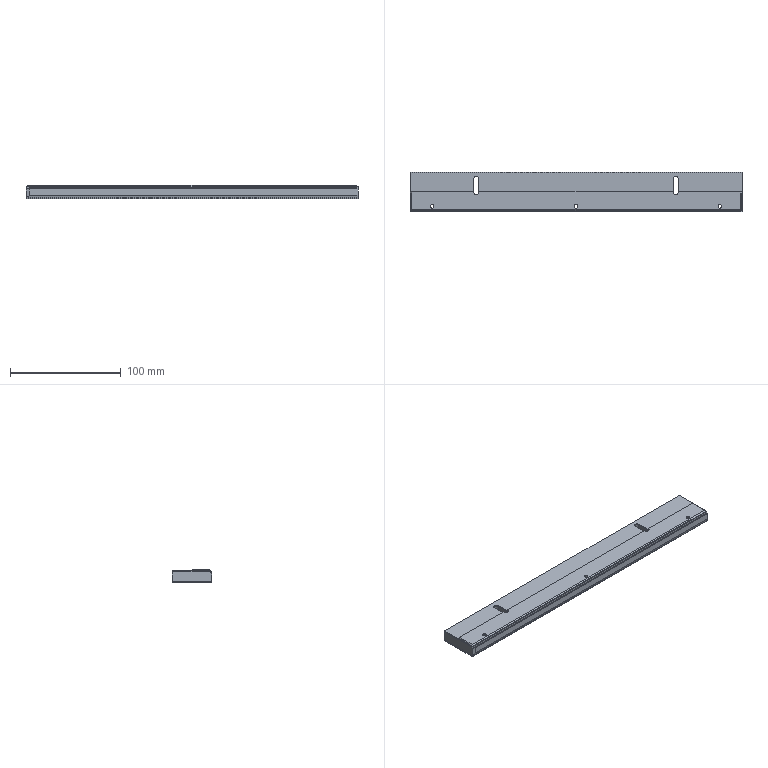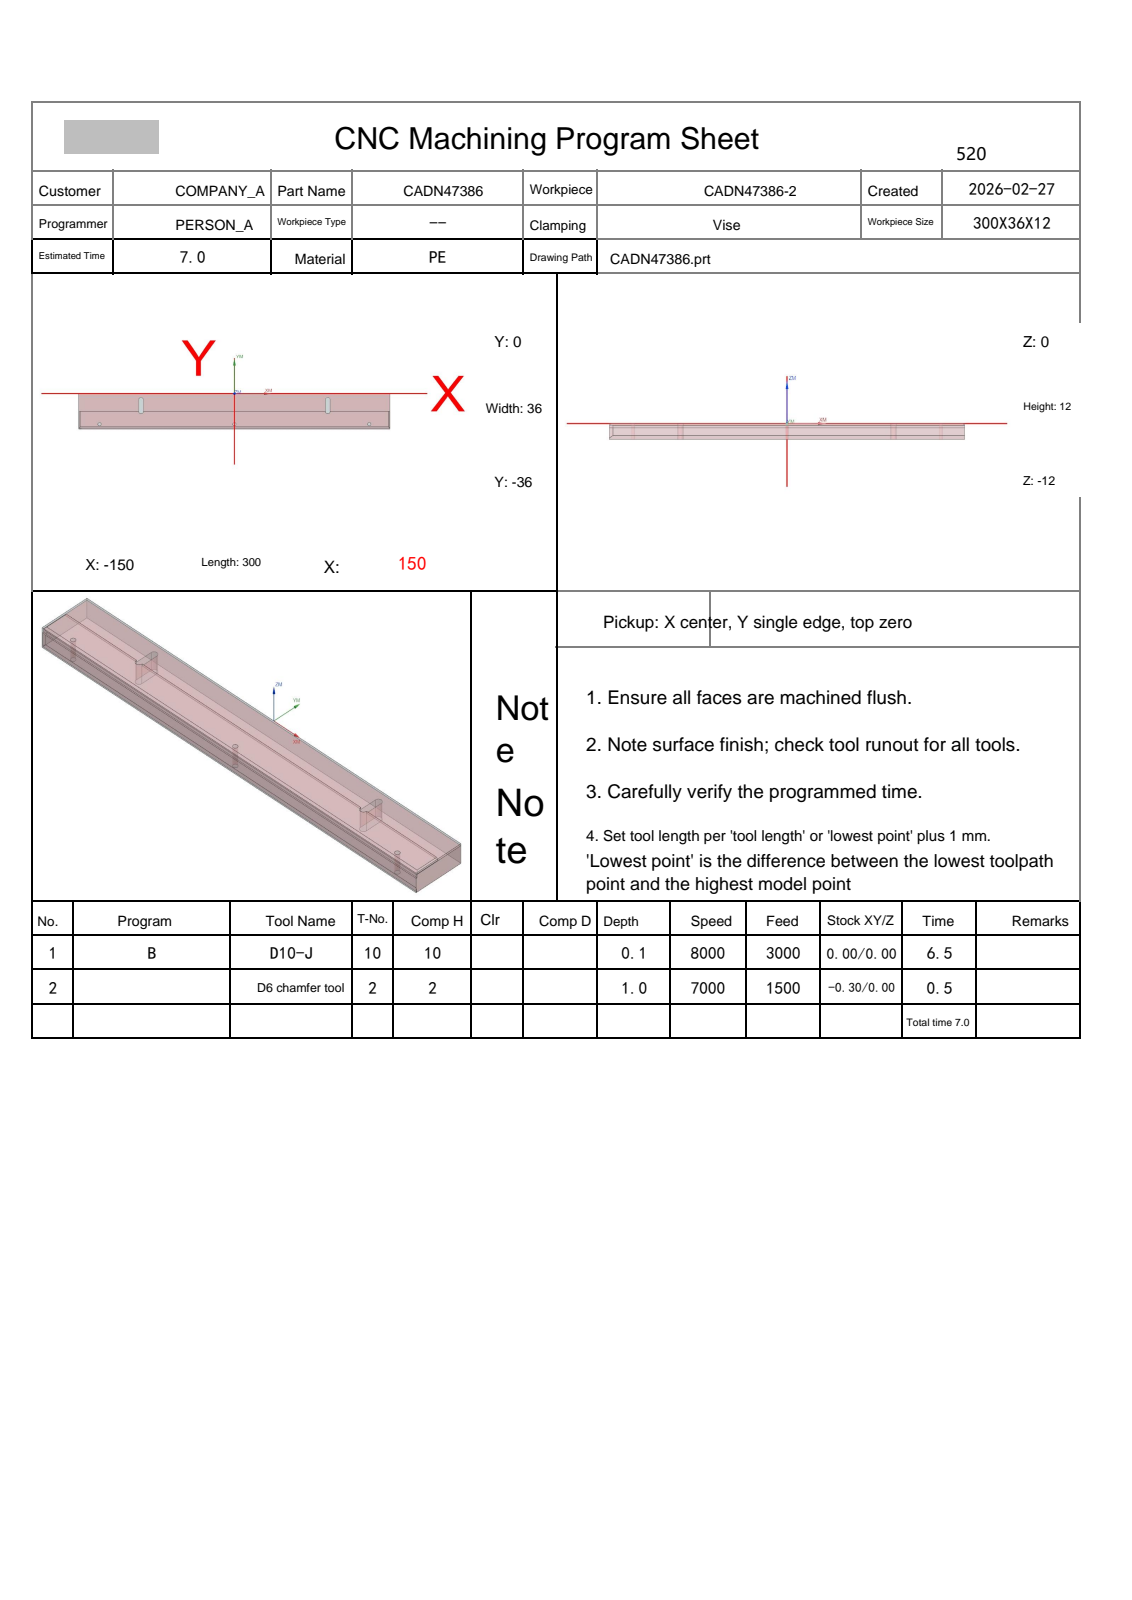NC program | NX | posted by the shop | part box 300 x 36 x 12 mm
Whole program:
%
O0001
(Machine time: 7.37 MIN)
(===Total Tool:2===)
(T10=D10-J  D=10.  R=0.   D-  H10 Z=0.    )
(T2=D6 chamfer tool   D=6.   R=0.   D-  H02 Z=-1.   )
G80 G90 G17 G49 G40
G91 G28 Z0
M01
N1 T10 M06
(D10-J  D=10. R=0. H=10 ce=0.20 di=0.10)
G00 G90 G54 X133.111 Y17. M03 S8000
G43 H10 Z50.
M08
Z4.02
G01 Z2.02 F3000.
X145.111 Y5.
X154.707 Y-4.596
G02 X155. Y-5.303 I-.707 J-.707
G01 Y-13.812
G02 X154.6 Y-14.212 I-.4 J0.0
X154.317 Y-14.095 I0.0 J.4
G01 X135.515 Y4.707
G03 X134.808 Y5. I-.707 J-.707
G01 X126.299
G03 X125.899 Y4.6 I0.0 J-.4
X126.016 Y4.317 I.4 J0.0
G01 X154.707 Y-24.374
G02 X155. Y-25.08 I-.707 J-.707
G01 Y-33.59
G02 X154.6 Y-33.99 I-.4 J0.0
X154.317 Y-33.873 I0.0 J.4
G01 X115.737 Y4.707
G03 X115.031 Y5. I-.707 J-.707
G01 X106.521
G03 X106.121 Y4.6 I0.0 J-.4
X106.238 Y4.317 I.4 J0.0
G01 X150.873 Y-40.317
G02 X150.99 Y-40.6 I-.283 J-.283
X150.59 Y-41. I-.4 J0.0
G01 X142.08
G02 X141.374 Y-40.707 I.001 J1.
G01 X95.959 Y4.707
G03 X95.253 Y5. I-.707 J-.707
G01 X86.743
G03 X86.343 Y4.6 I0.0 J-.4
X86.46 Y4.317 I.4 J0.0
G01 X131.095 Y-40.317
G02 X131.212 Y-40.6 I-.283 J-.283
X130.812 Y-41. I-.4 J0.0
G01 X122.303
G02 X121.596 Y-40.707 I.001 J1.
G01 X76.181 Y4.707
G03 X75.475 Y5. I-.707 J-.707
G01 X66.965
G03 X66.566 Y4.6 I0.0 J-.4
X66.683 Y4.317 I.4 J0.0
G01 X111.317 Y-40.317
G02 X111.434 Y-40.6 I-.283 J-.283
X111.035 Y-41. I-.4 J0.0
G01 X102.525
G02 X101.819 Y-40.707 I.001 J1.
G01 X56.404 Y4.707
G03 X55.697 Y5. I-.707 J-.707
G01 X47.188
G03 X46.788 Y4.6 I0.0 J-.4
X46.905 Y4.317 I.4 J0.0
G01 X91.54 Y-40.317
G02 X91.657 Y-40.6 I-.283 J-.283
X91.257 Y-41. I-.4 J0.0
G01 X82.747
G02 X82.041 Y-40.707 I.001 J1.
G01 X36.626 Y4.707
G03 X35.92 Y5. I-.707 J-.707
G01 X27.41
G03 X27.01 Y4.6 I0.0 J-.4
X27.127 Y4.317 I.4 J0.0
G01 X71.762 Y-40.317
G02 X71.879 Y-40.6 I-.283 J-.283
X71.479 Y-41. I-.4 J0.0
G01 X62.969
G02 X62.263 Y-40.707 I.001 J1.
G01 X16.848 Y4.707
G03 X16.142 Y5. I-.707 J-.707
G01 X7.632
G03 X7.232 Y4.6 I0.0 J-.4
X7.349 Y4.317 I.4 J0.0
G01 X51.984 Y-40.317
G02 X52.101 Y-40.6 I-.283 J-.283
X51.701 Y-41. I-.4 J0.0
G01 X43.191
G02 X42.485 Y-40.707 I.001 J1.
G01 X-2.93 Y4.707
G03 X-3.636 Y5. I-.707 J-.707
G01 X-12.146
G03 X-12.545 Y4.6 I0.0 J-.4
X-12.429 Y4.317 I.4 J0.0
G01 X32.206 Y-40.317
G02 X32.323 Y-40.6 I-.283 J-.283
X31.924 Y-41. I-.4 J0.0
G01 X23.414
G02 X22.707 Y-40.707 I.001 J1.
G01 X-22.707 Y4.707
G03 X-23.414 Y5. I-.707 J-.707
G01 X-31.924
G03 X-32.323 Y4.6 I0.0 J-.4
X-32.206 Y4.317 I.4 J0.0
G01 X12.429 Y-40.317
G02 X12.545 Y-40.6 I-.283 J-.283
X12.146 Y-41. I-.4 J0.0
G01 X3.636
G02 X2.93 Y-40.708 I.001 J1.
G01 X-42.485 Y4.707
G03 X-43.191 Y5. I-.707 J-.707
G01 X-51.701
G03 X-52.101 Y4.6 I0.0 J-.4
X-51.984 Y4.317 I.4 J0.0
G01 X-7.349 Y-40.317
G02 X-7.232 Y-40.6 I-.283 J-.283
X-7.632 Y-41. I-.4 J0.0
G01 X-16.142
G02 X-16.848 Y-40.708 I.001 J1.
G01 X-62.263 Y4.707
G03 X-62.969 Y5. I-.707 J-.707
G01 X-71.479
G03 X-71.879 Y4.6 I0.0 J-.4
X-71.762 Y4.317 I.4 J0.0
G01 X-27.127 Y-40.317
G02 X-27.01 Y-40.6 I-.283 J-.283
X-27.41 Y-41. I-.4 J0.0
G01 X-35.92
G02 X-36.626 Y-40.708 I.001 J1.
G01 X-82.041 Y4.707
G03 X-82.747 Y5. I-.707 J-.707
G01 X-91.257
G03 X-91.657 Y4.6 I0.0 J-.4
X-91.54 Y4.317 I.4 J0.0
G01 X-46.905 Y-40.317
G02 X-46.788 Y-40.6 I-.283 J-.283
X-47.188 Y-41. I-.4 J0.0
G01 X-55.697
G02 X-56.404 Y-40.708 I.001 J1.
G01 X-101.819 Y4.707
G03 X-102.525 Y5. I-.707 J-.707
G01 X-111.035
G03 X-111.434 Y4.6 I0.0 J-.4
X-111.317 Y4.317 I.4 J0.0
G01 X-66.683 Y-40.317
G02 X-66.566 Y-40.6 I-.283 J-.283
X-66.965 Y-41. I-.4 J0.0
G01 X-75.475
G02 X-76.181 Y-40.707 I.001 J1.
G01 X-121.596 Y4.707
G03 X-122.303 Y5. I-.707 J-.707
G01 X-130.812
G03 X-131.212 Y4.6 I0.0 J-.4
X-131.095 Y4.317 I.4 J0.0
G01 X-86.46 Y-40.317
G02 X-86.343 Y-40.6 I-.283 J-.283
X-86.743 Y-41. I-.4 J0.0
G01 X-95.253
G02 X-95.959 Y-40.707 I.001 J1.
G01 X-141.374 Y4.707
G03 X-142.08 Y5. I-.707 J-.707
G01 X-150.59
G03 X-150.99 Y4.6 I0.0 J-.4
X-150.873 Y4.317 I.4 J0.0
G01 X-106.238 Y-40.317
G02 X-106.121 Y-40.6 I-.283 J-.283
X-106.521 Y-41. I-.4 J0.0
G01 X-115.031
G02 X-115.737 Y-40.707 I.001 J1.
G01 X-154.317 Y-2.127
G03 X-154.6 Y-2.01 I-.283 J-.283
X-155. Y-2.41 I0.0 J-.4
G01 Y-10.92
G03 X-154.707 Y-11.626 I1. J.001
G01 X-126.016 Y-40.317
G02 X-125.899 Y-40.6 I-.283 J-.283
X-126.299 Y-41. I-.4 J0.0
G01 X-134.808
G02 X-135.515 Y-40.707 I0.0 J1.
G01 X-154.317 Y-21.905
G03 X-154.6 Y-21.788 I-.283 J-.283
X-155. Y-22.188 I0.0 J-.4
G01 Y-30.697
G03 X-154.707 Y-31.404 I1. J0.0
G01 X-145.111 Y-41.
X-133.111 Y-53.
Z4.02
G00 Z5.5
X167. Y-16.889
Z3.54
G01 Z1.54
X155. Y-4.889
X145.404 Y4.707
G03 X144.697 Y5. I-.707 J-.707
G01 X136.188
G03 X135.788 Y4.6 I0.0 J-.4
X135.905 Y4.317 I.4 J0.0
G01 X154.707 Y-14.485
G02 X155. Y-15.192 I-.707 J-.707
G01 Y-23.701
G02 X154.6 Y-24.101 I-.4 J0.0
X154.317 Y-23.984 I0.0 J.4
G01 X125.626 Y4.707
G03 X124.92 Y5. I-.707 J-.707
G01 X116.41
G03 X116.01 Y4.6 I0.0 J-.4
X116.127 Y4.317 I.4 J0.0
G01 X154.707 Y-34.263
G02 X155. Y-34.969 I-.707 J-.707
G01 Y-40.
G02 X154. Y-41. I-1. J0.0
G01 X151.969
G02 X151.263 Y-40.708 I.001 J1.
G01 X105.848 Y4.707
G03 X105.142 Y5. I-.707 J-.707
G01 X96.632
G03 X96.232 Y4.6 I0.0 J-.4
X96.349 Y4.317 I.4 J0.0
G01 X140.984 Y-40.317
G02 X141.101 Y-40.6 I-.283 J-.283
X140.701 Y-41. I-.4 J0.0
G01 X132.191
G02 X131.485 Y-40.707 I.001 J1.
G01 X86.07 Y4.707
G03 X85.364 Y5. I-.707 J-.707
G01 X76.854
G03 X76.455 Y4.6 I0.0 J-.4
X76.571 Y4.317 I.4 J0.0
G01 X121.206 Y-40.317
G02 X121.323 Y-40.6 I-.283 J-.283
X120.923 Y-41. I-.4 J0.0
G01 X112.414
G02 X111.708 Y-40.708 I.001 J1.
G01 X66.293 Y4.707
G03 X65.586 Y5. I-.707 J-.707
G01 X57.076
G03 X56.677 Y4.6 I0.0 J-.4
X56.794 Y4.317 I.4 J0.0
G01 X101.429 Y-40.317
G02 X101.545 Y-40.6 I-.283 J-.283
X101.146 Y-41. I-.4 J0.0
G01 X92.636
G02 X91.93 Y-40.707 I.001 J1.
G01 X46.515 Y4.707
G03 X45.809 Y5. I-.707 J-.707
G01 X37.299
G03 X36.899 Y4.6 I0.0 J-.4
X37.016 Y4.317 I.4 J0.0
G01 X81.651 Y-40.317
G02 X81.768 Y-40.6 I-.283 J-.283
X81.368 Y-41. I-.4 J0.0
G01 X72.858
G02 X72.152 Y-40.707 I.001 J1.
G01 X26.737 Y4.707
G03 X26.031 Y5. I-.707 J-.707
G01 X17.521
G03 X17.121 Y4.6 I0.0 J-.4
X17.238 Y4.317 I.4 J0.0
G01 X61.873 Y-40.317
G02 X61.99 Y-40.6 I-.283 J-.283
X61.59 Y-41. I-.4 J0.0
G01 X53.08
G02 X52.374 Y-40.707 I.001 J1.
G01 X6.959 Y4.707
G03 X6.253 Y5. I-.707 J-.707
G01 X-2.257
G03 X-2.657 Y4.6 I0.0 J-.4
X-2.54 Y4.317 I.4 J0.0
G01 X42.095 Y-40.317
G02 X42.212 Y-40.6 I-.283 J-.283
X41.812 Y-41. I-.4 J0.0
G01 X33.303
G02 X32.596 Y-40.707 I.001 J1.
G01 X-12.819 Y4.707
G03 X-13.525 Y5. I-.707 J-.707
G01 X-22.035
G03 X-22.434 Y4.6 I0.0 J-.4
X-22.317 Y4.317 I.4 J0.0
G01 X22.317 Y-40.317
G02 X22.434 Y-40.6 I-.283 J-.283
X22.035 Y-41. I-.4 J0.0
G01 X13.525
G02 X12.819 Y-40.708 I.001 J1.
G01 X-32.596 Y4.707
G03 X-33.303 Y5. I-.707 J-.707
G01 X-41.812
G03 X-42.212 Y4.6 I0.0 J-.4
X-42.095 Y4.317 I.4 J0.0
G01 X2.54 Y-40.317
G02 X2.657 Y-40.6 I-.283 J-.283
X2.257 Y-41. I-.4 J0.0
G01 X-6.253
G02 X-6.959 Y-40.708 I.001 J1.
G01 X-52.374 Y4.707
G03 X-53.08 Y5. I-.707 J-.707
G01 X-61.59
G03 X-61.99 Y4.6 I0.0 J-.4
X-61.873 Y4.317 I.4 J0.0
G01 X-17.238 Y-40.317
G02 X-17.121 Y-40.6 I-.283 J-.283
X-17.521 Y-41. I-.4 J0.0
G01 X-26.031
G02 X-26.737 Y-40.707 I.001 J1.
G01 X-72.152 Y4.707
G03 X-72.858 Y5. I-.707 J-.707
G01 X-81.368
G03 X-81.768 Y4.6 I0.0 J-.4
X-81.651 Y4.317 I.4 J0.0
G01 X-37.016 Y-40.317
G02 X-36.899 Y-40.6 I-.283 J-.283
X-37.299 Y-41. I-.4 J0.0
G01 X-45.809
G02 X-46.515 Y-40.708 I.001 J1.
G01 X-91.93 Y4.707
G03 X-92.636 Y5. I-.707 J-.707
G01 X-101.146
G03 X-101.545 Y4.6 I0.0 J-.4
X-101.429 Y4.317 I.4 J0.0
G01 X-56.794 Y-40.317
G02 X-56.677 Y-40.6 I-.283 J-.283
X-57.077 Y-41. I-.4 J0.0
G01 X-65.586
G02 X-66.293 Y-40.707 I.001 J1.
G01 X-111.707 Y4.707
G03 X-112.414 Y5. I-.707 J-.707
G01 X-120.924
G03 X-121.323 Y4.6 I0.0 J-.4
X-121.206 Y4.317 I.4 J0.0
G01 X-76.572 Y-40.317
G02 X-76.455 Y-40.6 I-.283 J-.283
X-76.854 Y-41. I-.4 J0.0
G01 X-85.364
G02 X-86.07 Y-40.707 I.001 J1.
G01 X-131.485 Y4.707
G03 X-132.191 Y5. I-.707 J-.707
G01 X-140.701
G03 X-141.101 Y4.6 I0.0 J-.4
X-140.984 Y4.317 I.4 J0.0
G01 X-96.349 Y-40.317
G02 X-96.232 Y-40.6 I-.283 J-.283
X-96.632 Y-41. I-.4 J0.0
G01 X-105.142
G02 X-105.848 Y-40.708 I.001 J1.
G01 X-151.263 Y4.707
G03 X-151.969 Y5. I-.707 J-.707
G01 X-154.
G03 X-155. Y4. I0.0 J-1.
G01 Y-1.031
G03 X-154.707 Y-1.737 I1. J.001
G01 X-116.127 Y-40.317
G02 X-116.01 Y-40.6 I-.283 J-.283
X-116.41 Y-41. I-.4 J0.0
G01 X-124.92
G02 X-125.626 Y-40.707 I.001 J1.
G01 X-154.317 Y-12.016
G03 X-154.6 Y-11.899 I-.283 J-.283
X-155. Y-12.299 I0.0 J-.4
G01 Y-20.808
G03 X-154.707 Y-21.515 I1. J0.0
G01 X-135.905 Y-40.317
G02 X-135.788 Y-40.6 I-.283 J-.283
X-136.188 Y-41. I-.4 J0.0
G01 X-144.697
G02 X-145.404 Y-40.707 I0.0 J1.
G01 X-155. Y-31.111
X-167. Y-19.111
Z3.54
G00 Z5.02
X167. Y-16.889
Z3.06
G01 Z1.06
X155. Y-4.889
X145.404 Y4.707
G03 X144.697 Y5. I-.707 J-.707
G01 X136.188
G03 X135.788 Y4.6 I0.0 J-.4
X135.905 Y4.317 I.4 J0.0
G01 X154.707 Y-14.485
G02 X155. Y-15.192 I-.707 J-.707
G01 Y-23.701
G02 X154.6 Y-24.101 I-.4 J0.0
X154.317 Y-23.984 I0.0 J.4
G01 X125.626 Y4.707
G03 X124.92 Y5. I-.707 J-.707
G01 X116.41
G03 X116.01 Y4.6 I0.0 J-.4
X116.127 Y4.317 I.4 J0.0
G01 X154.707 Y-34.263
G02 X155. Y-34.969 I-.707 J-.707
G01 Y-40.
G02 X154. Y-41. I-1. J0.0
G01 X151.969
G02 X151.263 Y-40.708 I.001 J1.
G01 X105.848 Y4.707
G03 X105.142 Y5. I-.707 J-.707
G01 X96.632
G03 X96.232 Y4.6 I0.0 J-.4
X96.349 Y4.317 I.4 J0.0
G01 X140.984 Y-40.317
G02 X141.101 Y-40.6 I-.283 J-.283
X140.701 Y-41. I-.4 J0.0
G01 X132.191
G02 X131.485 Y-40.707 I.001 J1.
G01 X86.07 Y4.707
G03 X85.364 Y5. I-.707 J-.707
G01 X76.854
G03 X76.455 Y4.6 I0.0 J-.4
X76.571 Y4.317 I.4 J0.0
G01 X121.206 Y-40.317
G02 X121.323 Y-40.6 I-.283 J-.283
X120.923 Y-41. I-.4 J0.0
G01 X112.414
G02 X111.708 Y-40.708 I.001 J1.
G01 X66.293 Y4.707
G03 X65.586 Y5. I-.707 J-.707
G01 X57.076
G03 X56.677 Y4.6 I0.0 J-.4
X56.794 Y4.317 I.4 J0.0
G01 X101.429 Y-40.317
G02 X101.545 Y-40.6 I-.283 J-.283
X101.146 Y-41. I-.4 J0.0
G01 X92.636
G02 X91.93 Y-40.707 I.001 J1.
G01 X46.515 Y4.707
G03 X45.809 Y5. I-.707 J-.707
G01 X37.299
G03 X36.899 Y4.6 I0.0 J-.4
X37.016 Y4.317 I.4 J0.0
G01 X81.651 Y-40.317
G02 X81.768 Y-40.6 I-.283 J-.283
X81.368 Y-41. I-.4 J0.0
G01 X72.858
G02 X72.152 Y-40.707 I.001 J1.
G01 X26.737 Y4.707
G03 X26.031 Y5. I-.707 J-.707
G01 X17.521
G03 X17.121 Y4.6 I0.0 J-.4
X17.238 Y4.317 I.4 J0.0
G01 X61.873 Y-40.317
G02 X61.99 Y-40.6 I-.283 J-.283
X61.59 Y-41. I-.4 J0.0
G01 X53.08
G02 X52.374 Y-40.707 I.001 J1.
G01 X6.959 Y4.707
G03 X6.253 Y5. I-.707 J-.707
G01 X-2.257
G03 X-2.657 Y4.6 I0.0 J-.4
X-2.54 Y4.317 I.4 J0.0
G01 X42.095 Y-40.317
G02 X42.212 Y-40.6 I-.283 J-.283
X41.812 Y-41. I-.4 J0.0
G01 X33.303
G02 X32.596 Y-40.707 I.001 J1.
G01 X-12.819 Y4.707
G03 X-13.525 Y5. I-.707 J-.707
G01 X-22.035
G03 X-22.434 Y4.6 I0.0 J-.4
X-22.317 Y4.317 I.4 J0.0
G01 X22.317 Y-40.317
G02 X22.434 Y-40.6 I-.283 J-.283
X22.035 Y-41. I-.4 J0.0
G01 X13.525
G02 X12.819 Y-40.708 I.001 J1.
G01 X-32.596 Y4.707
G03 X-33.303 Y5. I-.707 J-.707
G01 X-41.812
G03 X-42.212 Y4.6 I0.0 J-.4
X-42.095 Y4.317 I.4 J0.0
G01 X2.54 Y-40.317
G02 X2.657 Y-40.6 I-.283 J-.283
X2.257 Y-41. I-.4 J0.0
G01 X-6.253
G02 X-6.959 Y-40.708 I.001 J1.
G01 X-52.374 Y4.707
G03 X-53.08 Y5. I-.707 J-.707
G01 X-61.59
G03 X-61.99 Y4.6 I0.0 J-.4
X-61.873 Y4.317 I.4 J0.0
G01 X-17.238 Y-40.317
G02 X-17.121 Y-40.6 I-.283 J-.283
X-17.521 Y-41. I-.4 J0.0
G01 X-26.031
G02 X-26.737 Y-40.707 I.001 J1.
G01 X-72.152 Y4.707
G03 X-72.858 Y5. I-.707 J-.707
G01 X-81.368
G03 X-81.768 Y4.6 I0.0 J-.4
X-81.651 Y4.317 I.4 J0.0
G01 X-37.016 Y-40.317
G02 X-36.899 Y-40.6 I-.283 J-.283
X-37.299 Y-41. I-.4 J0.0
G01 X-45.809
G02 X-46.515 Y-40.708 I.001 J1.
G01 X-91.93 Y4.707
G03 X-92.636 Y5. I-.707 J-.707
G01 X-101.146
G03 X-101.545 Y4.6 I0.0 J-.4
X-101.429 Y4.317 I.4 J0.0
G01 X-56.794 Y-40.317
G02 X-56.677 Y-40.6 I-.283 J-.283
X-57.077 Y-41. I-.4 J0.0
G01 X-65.586
G02 X-66.293 Y-40.707 I.001 J1.
G01 X-111.707 Y4.707
G03 X-112.414 Y5. I-.707 J-.707
G01 X-120.924
G03 X-121.323 Y4.6 I0.0 J-.4
X-121.206 Y4.317 I.4 J0.0
G01 X-76.572 Y-40.317
G02 X-76.455 Y-40.6 I-.283 J-.283
X-76.854 Y-41. I-.4 J0.0
G01 X-85.364
G02 X-86.07 Y-40.707 I.001 J1.
G01 X-131.485 Y4.707
G03 X-132.191 Y5. I-.707 J-.707
G01 X-140.701
G03 X-141.101 Y4.6 I0.0 J-.4
X-140.984 Y4.317 I.4 J0.0
G01 X-96.349 Y-40.317
G02 X-96.232 Y-40.6 I-.283 J-.283
X-96.632 Y-41. I-.4 J0.0
G01 X-105.142
G02 X-105.848 Y-40.708 I.001 J1.
G01 X-151.263 Y4.707
G03 X-151.969 Y5. I-.707 J-.707
G01 X-154.
G03 X-155. Y4. I0.0 J-1.
G01 Y-1.031
G03 X-154.707 Y-1.737 I1. J.001
G01 X-116.127 Y-40.317
G02 X-116.01 Y-40.6 I-.283 J-.283
X-116.41 Y-41. I-.4 J0.0
G01 X-124.92
G02 X-125.626 Y-40.707 I.001 J1.
G01 X-154.317 Y-12.016
G03 X-154.6 Y-11.899 I-.283 J-.283
X-155. Y-12.299 I0.0 J-.4
G01 Y-20.808
G03 X-154.707 Y-21.515 I1. J0.0
G01 X-135.905 Y-40.317
G02 X-135.788 Y-40.6 I-.283 J-.283
X-136.188 Y-41. I-.4 J0.0
G01 X-144.697
G02 X-145.404 Y-40.707 I0.0 J1.
G01 X-155. Y-31.111
X-167. Y-19.111
Z3.06
G00 Z4.54
X167. Y-16.889
Z2.58
G01 Z.58
X155. Y-4.889
X145.404 Y4.707
G03 X144.697 Y5. I-.707 J-.707
G01 X136.188
G03 X135.788 Y4.6 I0.0 J-.4
X135.905 Y4.317 I.4 J0.0
G01 X154.707 Y-14.485
G02 X155. Y-15.192 I-.707 J-.707
G01 Y-23.701
G02 X154.6 Y-24.101 I-.4 J0.0
X154.317 Y-23.984 I0.0 J.4
G01 X125.626 Y4.707
G03 X124.92 Y5. I-.707 J-.707
G01 X116.41
G03 X116.01 Y4.6 I0.0 J-.4
X116.127 Y4.317 I.4 J0.0
G01 X154.707 Y-34.263
G02 X155. Y-34.969 I-.707 J-.707
G01 Y-40.
G02 X154. Y-41. I-1. J0.0
G01 X151.969
G02 X151.263 Y-40.708 I.001 J1.
G01 X105.848 Y4.707
G03 X105.142 Y5. I-.707 J-.707
G01 X96.632
G03 X96.232 Y4.6 I0.0 J-.4
X96.349 Y4.317 I.4 J0.0
G01 X140.984 Y-40.317
G02 X141.101 Y-40.6 I-.283 J-.283
X140.701 Y-41. I-.4 J0.0
G01 X132.191
G02 X131.485 Y-40.707 I.001 J1.
G01 X86.07 Y4.707
G03 X85.364 Y5. I-.707 J-.707
G01 X76.854
G03 X76.455 Y4.6 I0.0 J-.4
X76.571 Y4.317 I.4 J0.0
G01 X121.206 Y-40.317
G02 X121.323 Y-40.6 I-.283 J-.283
X120.923 Y-41. I-.4 J0.0
G01 X112.414
G02 X111.708 Y-40.708 I.001 J1.
G01 X66.293 Y4.707
G03 X65.586 Y5. I-.707 J-.707
G01 X57.076
G03 X56.677 Y4.6 I0.0 J-.4
X56.794 Y4.317 I.4 J0.0
G01 X101.429 Y-40.317
G02 X101.545 Y-40.6 I-.283 J-.283
X101.146 Y-41. I-.4 J0.0
G01 X92.636
G02 X91.93 Y-40.707 I.001 J1.
G01 X46.515 Y4.707
G03 X45.809 Y5. I-.707 J-.707
G01 X37.299
G03 X36.899 Y4.6 I0.0 J-.4
X37.016 Y4.317 I.4 J0.0
G01 X81.651 Y-40.317
G02 X81.768 Y-40.6 I-.283 J-.283
X81.368 Y-41. I-.4 J0.0
G01 X72.858
G02 X72.152 Y-40.707 I.001 J1.
G01 X26.737 Y4.707
G03 X26.031 Y5. I-.707 J-.707
G01 X17.521
G03 X17.121 Y4.6 I0.0 J-.4
X17.238 Y4.317 I.4 J0.0
G01 X61.873 Y-40.317
G02 X61.99 Y-40.6 I-.283 J-.283
X61.59 Y-41. I-.4 J0.0
G01 X53.08
G02 X52.374 Y-40.707 I.001 J1.
G01 X6.959 Y4.707
G03 X6.253 Y5. I-.707 J-.707
G01 X-2.257
G03 X-2.657 Y4.6 I0.0 J-.4
X-2.54 Y4.317 I.4 J0.0
G01 X42.095 Y-40.317
G02 X42.212 Y-40.6 I-.283 J-.283
X41.812 Y-41. I-.4 J0.0
G01 X33.303
G02 X32.596 Y-40.707 I.001 J1.
G01 X-12.819 Y4.707
G03 X-13.525 Y5. I-.707 J-.707
G01 X-22.035
G03 X-22.434 Y4.6 I0.0 J-.4
X-22.317 Y4.317 I.4 J0.0
G01 X22.317 Y-40.317
G02 X22.434 Y-40.6 I-.283 J-.283
X22.035 Y-41. I-.4 J0.0
G01 X13.525
G02 X12.819 Y-40.708 I.001 J1.
G01 X-32.596 Y4.707
G03 X-33.303 Y5. I-.707 J-.707
G01 X-41.812
G03 X-42.212 Y4.6 I0.0 J-.4
X-42.095 Y4.317 I.4 J0.0
G01 X2.54 Y-40.317
G02 X2.657 Y-40.6 I-.283 J-.283
X2.257 Y-41. I-.4 J0.0
G01 X-6.253
G02 X-6.959 Y-40.708 I.001 J1.
G01 X-52.374 Y4.707
G03 X-53.08 Y5. I-.707 J-.707
G01 X-61.59
G03 X-61.99 Y4.6 I0.0 J-.4
X-61.873 Y4.317 I.4 J0.0
G01 X-17.238 Y-40.317
G02 X-17.121 Y-40.6 I-.283 J-.283
X-17.521 Y-41. I-.4 J0.0
G01 X-26.031
G02 X-26.737 Y-40.707 I.001 J1.
G01 X-72.152 Y4.707
G03 X-72.858 Y5. I-.707 J-.707
G01 X-81.368
G03 X-81.768 Y4.6 I0.0 J-.4
X-81.651 Y4.317 I.4 J0.0
G01 X-37.016 Y-40.317
G02 X-36.899 Y-40.6 I-.283 J-.283
X-37.299 Y-41. I-.4 J0.0
G01 X-45.809
G02 X-46.515 Y-40.708 I.001 J1.
G01 X-91.93 Y4.707
G03 X-92.636 Y5. I-.707 J-.707
G01 X-101.146
G03 X-101.545 Y4.6 I0.0 J-.4
X-101.429 Y4.317 I.4 J0.0
G01 X-56.794 Y-40.317
G02 X-56.677 Y-40.6 I-.283 J-.283
X-57.077 Y-41. I-.4 J0.0
G01 X-65.586
G02 X-66.293 Y-40.707 I.001 J1.
G01 X-111.707 Y4.707
G03 X-112.414 Y5. I-.707 J-.707
G01 X-120.924
G03 X-121.323 Y4.6 I0.0 J-.4
X-121.206 Y4.317 I.4 J0.0
G01 X-76.572 Y-40.317
G02 X-76.455 Y-40.6 I-.283 J-.283
X-76.854 Y-41. I-.4 J0.0
G01 X-85.364
G02 X-86.07 Y-40.707 I.001 J1.
G01 X-131.485 Y4.707
G03 X-132.191 Y5. I-.707 J-.707
G01 X-140.701
G03 X-141.101 Y4.6 I0.0 J-.4
X-140.984 Y4.317 I.4 J0.0
G01 X-96.349 Y-40.317
G02 X-96.232 Y-40.6 I-.283 J-.283
X-96.632 Y-41. I-.4 J0.0
G01 X-105.142
G02 X-105.848 Y-40.708 I.001 J1.
G01 X-151.263 Y4.707
G03 X-151.969 Y5. I-.707 J-.707
G01 X-154.
G03 X-155. Y4. I0.0 J-1.
G01 Y-1.031
G03 X-154.707 Y-1.737 I1. J.001
G01 X-116.127 Y-40.317
G02 X-116.01 Y-40.6 I-.283 J-.283
X-116.41 Y-41. I-.4 J0.0
G01 X-124.92
G02 X-125.626 Y-40.707 I.001 J1.
G01 X-154.317 Y-12.016
G03 X-154.6 Y-11.899 I-.283 J-.283
X-155. Y-12.299 I0.0 J-.4
G01 Y-20.808
G03 X-154.707 Y-21.515 I1. J0.0
G01 X-135.905 Y-40.317
G02 X-135.788 Y-40.6 I-.283 J-.283
X-136.188 Y-41. I-.4 J0.0
G01 X-144.697
G02 X-145.404 Y-40.707 I0.0 J1.
G01 X-155. Y-31.111
X-167. Y-19.111
Z2.58
G00 Z4.06
X167. Y-16.889
Z2.1
G01 Z.1
X155. Y-4.889
X145.404 Y4.707
G03 X144.697 Y5. I-.707 J-.707
G01 X136.188
G03 X135.788 Y4.6 I0.0 J-.4
X135.905 Y4.317 I.4 J0.0
G01 X154.707 Y-14.485
G02 X155. Y-15.192 I-.707 J-.707
G01 Y-23.701
G02 X154.6 Y-24.101 I-.4 J0.0
X154.317 Y-23.984 I0.0 J.4
G01 X125.626 Y4.707
G03 X124.92 Y5. I-.707 J-.707
G01 X116.41
G03 X116.01 Y4.6 I0.0 J-.4
X116.127 Y4.317 I.4 J0.0
G01 X154.707 Y-34.263
G02 X155. Y-34.969 I-.707 J-.707
G01 Y-40.
G02 X154. Y-41. I-1. J0.0
G01 X151.969
G02 X151.263 Y-40.708 I.001 J1.
G01 X105.848 Y4.707
G03 X105.142 Y5. I-.707 J-.707
G01 X96.632
G03 X96.232 Y4.6 I0.0 J-.4
X96.349 Y4.317 I.4 J0.0
G01 X140.984 Y-40.317
G02 X141.101 Y-40.6 I-.283 J-.283
X140.701 Y-41. I-.4 J0.0
G01 X132.191
G02 X131.485 Y-40.707 I.001 J1.
G01 X86.07 Y4.707
G03 X85.364 Y5. I-.707 J-.707
G01 X76.854
G03 X76.455 Y4.6 I0.0 J-.4
X76.571 Y4.317 I.4 J0.0
G01 X121.206 Y-40.317
G02 X121.323 Y-40.6 I-.283 J-.283
X120.923 Y-41. I-.4 J0.0
G01 X112.414
G02 X111.708 Y-40.708 I.001 J1.
G01 X66.293 Y4.707
G03 X65.586 Y5. I-.707 J-.707
G01 X57.076
G03 X56.677 Y4.6 I0.0 J-.4
X56.794 Y4.317 I.4 J0.0
G01 X101.429 Y-40.317
G02 X101.545 Y-40.6 I-.283 J-.283
X101.146 Y-41. I-.4 J0.0
G01 X92.636
G02 X91.93 Y-40.707 I.001 J1.
G01 X46.515 Y4.707
G03 X45.809 Y5. I-.707 J-.707
G01 X37.299
G03 X36.899 Y4.6 I0.0 J-.4
X37.016 Y4.317 I.4 J0.0
G01 X81.651 Y-40.317
G02 X81.768 Y-40.6 I-.283 J-.283
X81.368 Y-41. I-.4 J0.0
G01 X72.858
G02 X72.152 Y-40.707 I.001 J1.
G01 X26.737 Y4.707
G03 X26.031 Y5. I-.707 J-.707
G01 X17.521
G03 X17.121 Y4.6 I0.0 J-.4
X17.238 Y4.317 I.4 J0.0
G01 X61.873 Y-40.317
G02 X61.99 Y-40.6 I-.283 J-.283
X61.59 Y-41. I-.4 J0.0
G01 X53.08
G02 X52.374 Y-40.707 I.001 J1.
G01 X6.959 Y4.707
G03 X6.253 Y5. I-.707 J-.707
G01 X-2.257
G03 X-2.657 Y4.6 I0.0 J-.4
X-2.54 Y4.317 I.4 J0.0
G01 X42.095 Y-40.317
G02 X42.212 Y-40.6 I-.283 J-.283
X41.812 Y-41. I-.4 J0.0
G01 X33.303
G02 X32.596 Y-40.707 I.001 J1.
G01 X-12.819 Y4.707
G03 X-13.525 Y5. I-.707 J-.707
G01 X-22.035
G03 X-22.434 Y4.6 I0.0 J-.4
X-22.317 Y4.317 I.4 J0.0
G01 X22.317 Y-40.317
G02 X22.434 Y-40.6 I-.283 J-.283
X22.035 Y-41. I-.4 J0.0
G01 X13.525
G02 X12.819 Y-40.708 I.001 J1.
G01 X-32.596 Y4.707
G03 X-33.303 Y5. I-.707 J-.707
G01 X-41.812
G03 X-42.212 Y4.6 I0.0 J-.4
X-42.095 Y4.317 I.4 J0.0
G01 X2.54 Y-40.317
G02 X2.657 Y-40.6 I-.283 J-.283
X2.257 Y-41. I-.4 J0.0
G01 X-6.253
G02 X-6.959 Y-40.708 I.001 J1.
G01 X-52.374 Y4.707
G03 X-53.08 Y5. I-.707 J-.707
G01 X-61.59
G03 X-61.99 Y4.6 I0.0 J-.4
X-61.873 Y4.317 I.4 J0.0
G01 X-17.238 Y-40.317
G02 X-17.121 Y-40.6 I-.283 J-.283
X-17.521 Y-41. I-.4 J0.0
G01 X-26.031
G02 X-26.737 Y-40.707 I.001 J1.
G01 X-72.152 Y4.707
G03 X-72.858 Y5. I-.707 J-.707
G01 X-81.368
G03 X-81.768 Y4.6 I0.0 J-.4
X-81.651 Y4.317 I.4 J0.0
G01 X-37.016 Y-40.317
G02 X-36.899 Y-40.6 I-.283 J-.283
X-37.299 Y-41. I-.4 J0.0
G01 X-45.809
G02 X-46.515 Y-40.708 I.001 J1.
G01 X-91.93 Y4.707
G03 X-92.636 Y5. I-.707 J-.707
G01 X-101.146
G03 X-101.545 Y4.6 I0.0 J-.4
X-101.429 Y4.317 I.4 J0.0
G01 X-56.794 Y-40.317
G02 X-56.677 Y-40.6 I-.283 J-.283
X-57.077 Y-41. I-.4 J0.0
G01 X-65.586
G02 X-66.293 Y-40.707 I.001 J1.
G01 X-111.707 Y4.707
G03 X-112.414 Y5. I-.707 J-.707
G01 X-120.924
G03 X-121.323 Y4.6 I0.0 J-.4
X-121.206 Y4.317 I.4 J0.0
G01 X-76.572 Y-40.317
G02 X-76.455 Y-40.6 I-.283 J-.283
X-76.854 Y-41. I-.4 J0.0
G01 X-85.364
G02 X-86.07 Y-40.707 I.001 J1.
G01 X-131.485 Y4.707
G03 X-132.191 Y5. I-.707 J-.707
G01 X-140.701
G03 X-141.101 Y4.6 I0.0 J-.4
X-140.984 Y4.317 I.4 J0.0
G01 X-96.349 Y-40.317
G02 X-96.232 Y-40.6 I-.283 J-.283
X-96.632 Y-41. I-.4 J0.0
G01 X-105.142
G02 X-105.848 Y-40.708 I.001 J1.
G01 X-151.263 Y4.707
G03 X-151.969 Y5. I-.707 J-.707
G01 X-154.
G03 X-155. Y4. I0.0 J-1.
G01 Y-1.031
G03 X-154.707 Y-1.737 I1. J.001
G01 X-116.127 Y-40.317
G02 X-116.01 Y-40.6 I-.283 J-.283
X-116.41 Y-41. I-.4 J0.0
G01 X-124.92
G02 X-125.626 Y-40.707 I.001 J1.
G01 X-154.317 Y-12.016
G03 X-154.6 Y-11.899 I-.283 J-.283
X-155. Y-12.299 I0.0 J-.4
G01 Y-20.808
G03 X-154.707 Y-21.515 I1. J0.0
G01 X-135.905 Y-40.317
G02 X-135.788 Y-40.6 I-.283 J-.283
X-136.188 Y-41. I-.4 J0.0
G01 X-144.697
G02 X-145.404 Y-40.707 I0.0 J1.
G01 X-155. Y-31.111
X-167. Y-19.111
Z2.1
G00 Z50.
G00 G90 X133.111 Y17. M03 S8000
Z50.
Z2.
G01 Z0.0 F1000.
X145.111 Y5.
X155. Y-4.889
Y-14.778
X135.222 Y5.
X125.333
X155. Y-24.667
Y-34.556
X115.444 Y5.
X105.556
X151.556 Y-41.
X141.667
X95.667 Y5.
X85.778
X131.778 Y-41.
X121.889
X75.889 Y5.
X66.
X112. Y-41.
X102.111
X56.111 Y5.
X46.222
X92.222 Y-41.
X82.333
X36.333 Y5.
X26.444
X72.444 Y-41.
X62.556
X16.556 Y5.
X6.667
X52.667 Y-41.
X42.778
X-3.222 Y5.
X-13.111
X32.889 Y-41.
X23.
X-23. Y5.
X-32.889
X13.111 Y-41.
X3.222
X-42.778 Y5.
X-52.667
X-6.667 Y-41.
X-16.556
X-62.556 Y5.
X-72.444
X-26.444 Y-41.
X-36.333
X-82.333 Y5.
X-92.222
X-46.222 Y-41.
X-56.111
X-102.111 Y5.
X-112.
X-66. Y-41.
X-75.889
X-121.889 Y5.
X-131.778
X-85.778 Y-41.
X-95.667
X-141.667 Y5.
X-151.556
X-105.556 Y-41.
X-115.444
X-155. Y-1.444
Y-11.333
X-125.333 Y-41.
X-135.222
X-155. Y-21.222
Y-31.111
X-145.111 Y-41.
X-133.111 Y-53.
Z2.
G00 Z50.
G91 G28 Z0.0
M05
M09
G91 G28 Z0.0
M01
N2 T02 M06
(D6 chamfer tool  D=6. R=0. H=02 ce=-0.30 di=0.00)
G00 G90 G54 X-141.657 Y-36.7 M03 S7000
G43 H02 Z50.
M08
Z2.5
G01 X-149.778 Z-.456 F1500.
X-149.977 Y-36.664 Z-.529
X-150.165 Y-36.589 Z-.603
X-150.334 Y-36.477 Z-.677
X-150.477 Y-36.334 Z-.751
X-150.589 Y-36.165 Z-.824
X-150.664 Y-35.977 Z-.898
X-150.7 Y-35.778 Z-.972
Y-35.7 Z-1.
Y-.3
G02 X-149.7 Y.7 I1. J0.0
G01 X149.7
G02 X150.7 Y-.3 I0.0 J-1.
G01 Y-35.7
G02 X149.7 Y-36.7 I-1. J0.0
G01 X-149.7
G02 X-150.7 Y-35.7 I0.0 J1.
G01 Y-35.2
Z1.5
G00 Z50.
M05
M09
G91 G28 Z0.0
G91 G28 Y0.0
M30
%